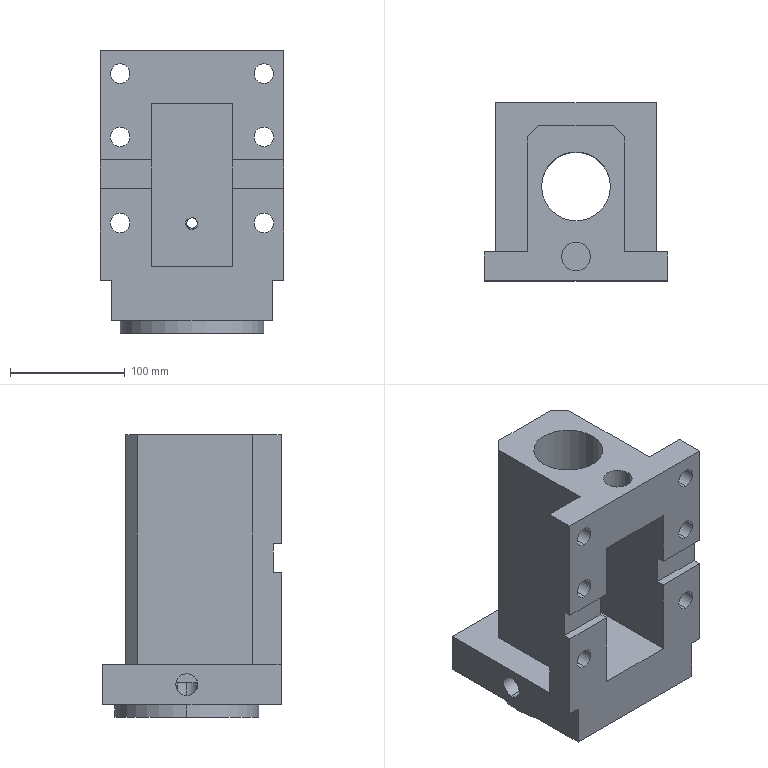Part | SolidWorks | features ICE 2, BaseBody 1 | 1 solid | 92 faces | box 160 x 155 x 246 mm | volume 1955692 mm3 | cylinder 49 | plane 39 | spline 3 | cone 1 | commonest cylinder face diameters 9 x15 17 x12 12 x8 19 x6 60 x4 25 x2